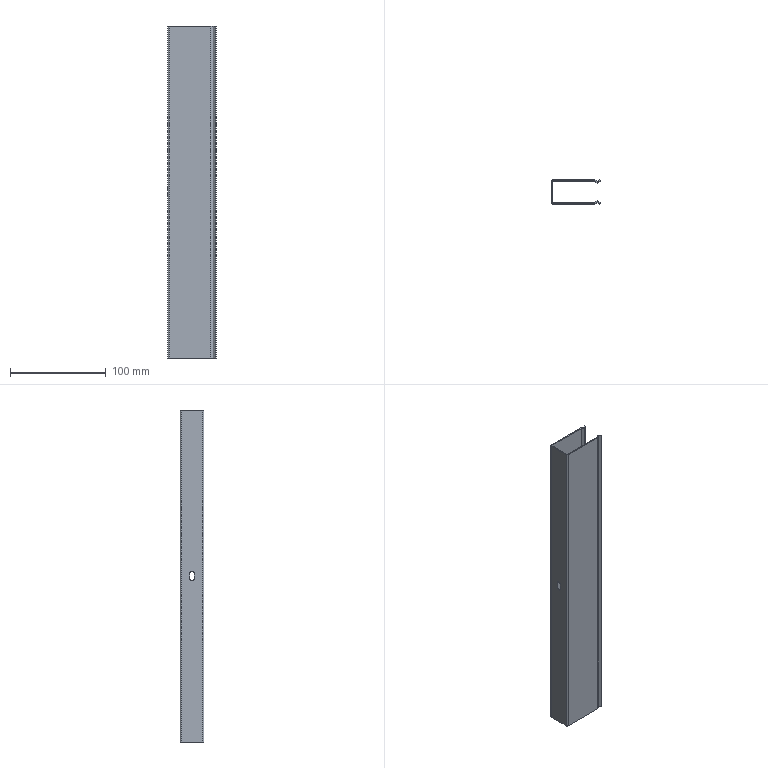Part | STEP file | Cable trough 5 | 1 solid | 27 faces | box 50.625 x 25 x 346 mm | volume 43498 mm3 | plane 20 | cylinder 7 | commonest cylinder face diameters 5 x3 1 x2 3 x2